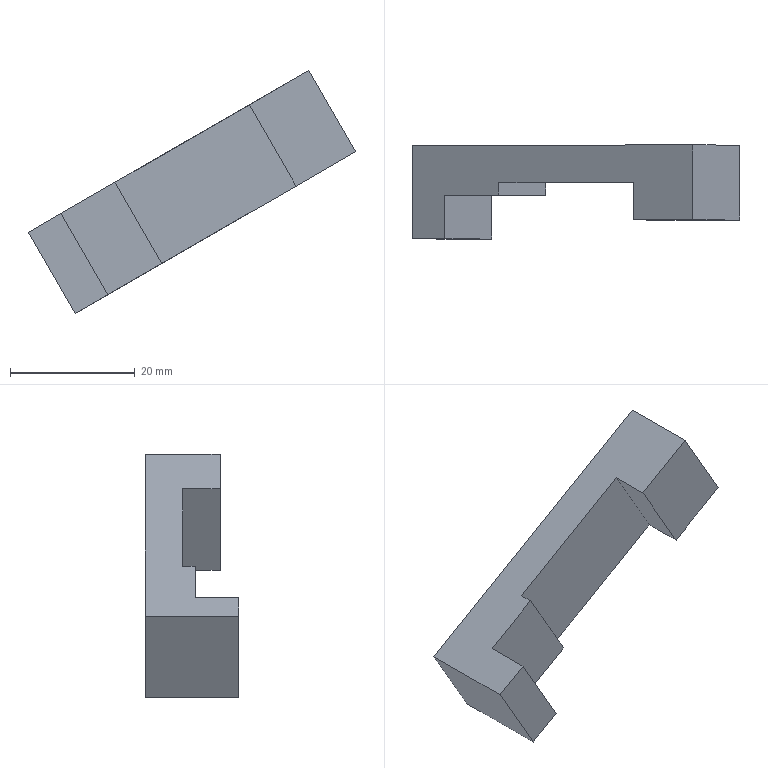Part | NX | features solid 2 | 1 solid | 12 faces | box 52.373 x 15 x 38.898 mm | volume 6763 mm3 | plane 12
STEP:
#1=CARTESIAN_POINT('',(16.962,778.,239.949));
#2=VERTEX_POINT('',#1);
#3=CARTESIAN_POINT('',(9.462,778.,252.94));
#4=VERTEX_POINT('',#3);
#5=CARTESIAN_POINT('',(16.962,778.,239.949));
#6=DIRECTION('',(0.5,0.,-0.866));
#7=VECTOR('',#6,1000.);
#8=LINE('',#5,#7);
#9=EDGE_CURVE('',#2,#4,#8,.F.);
#10=ORIENTED_EDGE('',*,*,#9,.T.);
#11=CARTESIAN_POINT('',(-12.029,778.,240.532));
#12=VERTEX_POINT('',#11);
#13=CARTESIAN_POINT('',(18.988,778.,258.44));
#14=DIRECTION('',(-0.866,0.,-0.5));
#15=VECTOR('',#14,1000.);
#16=LINE('',#13,#15);
#17=EDGE_CURVE('',#4,#12,#16,.T.);
#18=ORIENTED_EDGE('',*,*,#17,.T.);
#19=CARTESIAN_POINT('',(-4.529,778.,227.542));
#20=VERTEX_POINT('',#19);
#21=CARTESIAN_POINT('',(-4.529,778.,227.542));
#22=DIRECTION('',(-0.5,0.,0.866));
#23=VECTOR('',#22,1000.);
#24=LINE('',#21,#23);
#25=EDGE_CURVE('',#20,#12,#24,.T.);
#26=ORIENTED_EDGE('',*,*,#25,.F.);
#27=CARTESIAN_POINT('',(26.488,778.,245.449));
#28=DIRECTION('',(-0.866,0.,-0.5));
#29=VECTOR('',#28,1000.);
#30=LINE('',#27,#29);
#31=EDGE_CURVE('',#2,#20,#30,.T.);
#32=ORIENTED_EDGE('',*,*,#31,.F.);
#33=EDGE_LOOP('',(#10,#18,#26,#32));
#34=FACE_BOUND('',#33,.T.);
#35=CARTESIAN_POINT('',(11.488,778.,271.43));
#36=DIRECTION('',(0.,1.,0.));
#37=DIRECTION('',(-0.866,0.,-0.5));
#38=AXIS2_PLACEMENT_3D('',#35,#36,#37);
#39=PLANE('',#38);
#40=ADVANCED_FACE('',(#34),#39,.F.);
#41=CARTESIAN_POINT('',(26.488,784.,245.449));
#42=VERTEX_POINT('',#41);
#43=CARTESIAN_POINT('',(18.988,784.,258.44));
#44=VERTEX_POINT('',#43);
#45=CARTESIAN_POINT('',(11.488,784.,271.43));
#46=DIRECTION('',(0.5,0.,-0.866));
#47=VECTOR('',#46,1000.);
#48=LINE('',#45,#47);
#49=EDGE_CURVE('',#42,#44,#48,.F.);
#50=ORIENTED_EDGE('',*,*,#49,.F.);
#51=CARTESIAN_POINT('',(-18.385,784.,219.542));
#52=VERTEX_POINT('',#51);
#53=CARTESIAN_POINT('',(26.488,784.,245.449));
#54=DIRECTION('',(-0.866,0.,-0.5));
#55=VECTOR('',#54,1000.);
#56=LINE('',#53,#55);
#57=EDGE_CURVE('',#42,#52,#56,.T.);
#58=ORIENTED_EDGE('',*,*,#57,.T.);
#59=CARTESIAN_POINT('',(-25.885,784.,232.532));
#60=VERTEX_POINT('',#59);
#61=CARTESIAN_POINT('',(-33.385,784.,245.522));
#62=DIRECTION('',(-0.5,0.,0.866));
#63=VECTOR('',#62,1000.);
#64=LINE('',#61,#63);
#65=EDGE_CURVE('',#52,#60,#64,.T.);
#66=ORIENTED_EDGE('',*,*,#65,.T.);
#67=CARTESIAN_POINT('',(18.988,784.,258.44));
#68=DIRECTION('',(-0.866,0.,-0.5));
#69=VECTOR('',#68,1000.);
#70=LINE('',#67,#69);
#71=EDGE_CURVE('',#44,#60,#70,.T.);
#72=ORIENTED_EDGE('',*,*,#71,.F.);
#73=EDGE_LOOP('',(#50,#58,#66,#72));
#74=FACE_BOUND('',#73,.T.);
#75=CARTESIAN_POINT('',(11.488,784.,271.43));
#76=DIRECTION('',(0.,1.,0.));
#77=DIRECTION('',(-0.866,0.,-0.5));
#78=AXIS2_PLACEMENT_3D('',#75,#76,#77);
#79=PLANE('',#78);
#80=ADVANCED_FACE('',(#74),#79,.T.);
#81=ORIENTED_EDGE('',*,*,#65,.F.);
#82=CARTESIAN_POINT('',(-18.385,769.,219.542));
#83=VERTEX_POINT('',#82);
#84=CARTESIAN_POINT('',(-18.385,784.,219.542));
#85=DIRECTION('',(0.,1.,0.));
#86=VECTOR('',#85,1000.);
#87=LINE('',#84,#86);
#88=EDGE_CURVE('',#52,#83,#87,.F.);
#89=ORIENTED_EDGE('',*,*,#88,.T.);
#90=CARTESIAN_POINT('',(-25.885,769.,232.532));
#91=VERTEX_POINT('',#90);
#92=CARTESIAN_POINT('',(-18.385,769.,219.542));
#93=DIRECTION('',(-0.5,0.,0.866));
#94=VECTOR('',#93,1000.);
#95=LINE('',#92,#94);
#96=EDGE_CURVE('',#83,#91,#95,.T.);
#97=ORIENTED_EDGE('',*,*,#96,.T.);
#98=CARTESIAN_POINT('',(-25.885,784.,232.532));
#99=DIRECTION('',(0.,1.,0.));
#100=VECTOR('',#99,1000.);
#101=LINE('',#98,#100);
#102=EDGE_CURVE('',#60,#91,#101,.F.);
#103=ORIENTED_EDGE('',*,*,#102,.F.);
#104=EDGE_LOOP('',(#81,#89,#97,#103));
#105=FACE_BOUND('',#104,.T.);
#106=CARTESIAN_POINT('',(-33.385,784.,245.522));
#107=DIRECTION('',(-0.866,0.,-0.5));
#108=DIRECTION('',(0.,-1.,0.));
#109=AXIS2_PLACEMENT_3D('',#106,#107,#108);
#110=PLANE('',#109);
#111=ADVANCED_FACE('',(#105),#110,.T.);
#112=CARTESIAN_POINT('',(26.488,772.,245.449));
#113=VERTEX_POINT('',#112);
#114=CARTESIAN_POINT('',(26.488,784.,245.449));
#115=DIRECTION('',(0.,-1.,0.));
#116=VECTOR('',#115,1000.);
#117=LINE('',#114,#116);
#118=EDGE_CURVE('',#42,#113,#117,.T.);
#119=ORIENTED_EDGE('',*,*,#118,.F.);
#120=ORIENTED_EDGE('',*,*,#49,.T.);
#121=CARTESIAN_POINT('',(18.988,772.,258.44));
#122=VERTEX_POINT('',#121);
#123=CARTESIAN_POINT('',(18.988,784.,258.44));
#124=DIRECTION('',(0.,-1.,0.));
#125=VECTOR('',#124,1000.);
#126=LINE('',#123,#125);
#127=EDGE_CURVE('',#44,#122,#126,.T.);
#128=ORIENTED_EDGE('',*,*,#127,.T.);
#129=CARTESIAN_POINT('',(26.488,772.,245.449));
#130=DIRECTION('',(-0.5,0.,0.866));
#131=VECTOR('',#130,1000.);
#132=LINE('',#129,#131);
#133=EDGE_CURVE('',#113,#122,#132,.T.);
#134=ORIENTED_EDGE('',*,*,#133,.F.);
#135=EDGE_LOOP('',(#119,#120,#128,#134));
#136=FACE_BOUND('',#135,.T.);
#137=CARTESIAN_POINT('',(11.488,784.,271.43));
#138=DIRECTION('',(-0.866,0.,-0.5));
#139=DIRECTION('',(0.,-1.,0.));
#140=AXIS2_PLACEMENT_3D('',#137,#138,#139);
#141=PLANE('',#140);
#142=ADVANCED_FACE('',(#136),#141,.F.);
#143=CARTESIAN_POINT('',(-20.689,769.,235.532));
#144=VERTEX_POINT('',#143);
#145=CARTESIAN_POINT('',(-20.689,769.,235.532));
#146=DIRECTION('',(-0.866,0.,-0.5));
#147=VECTOR('',#146,1000.);
#148=LINE('',#145,#147);
#149=EDGE_CURVE('',#144,#91,#148,.T.);
#150=ORIENTED_EDGE('',*,*,#149,.F.);
#151=CARTESIAN_POINT('',(-20.689,776.,235.532));
#152=VERTEX_POINT('',#151);
#153=CARTESIAN_POINT('',(-20.689,778.,235.532));
#154=DIRECTION('',(0.,-1.,0.));
#155=VECTOR('',#154,1000.);
#156=LINE('',#153,#155);
#157=EDGE_CURVE('',#152,#144,#156,.T.);
#158=ORIENTED_EDGE('',*,*,#157,.F.);
#159=CARTESIAN_POINT('',(-12.029,776.,240.532));
#160=VERTEX_POINT('',#159);
#161=CARTESIAN_POINT('',(-12.029,776.,240.532));
#162=DIRECTION('',(-0.866,0.,-0.5));
#163=VECTOR('',#162,1000.);
#164=LINE('',#161,#163);
#165=EDGE_CURVE('',#160,#152,#164,.T.);
#166=ORIENTED_EDGE('',*,*,#165,.F.);
#167=CARTESIAN_POINT('',(-12.029,778.,240.532));
#168=DIRECTION('',(0.,-1.,0.));
#169=VECTOR('',#168,1000.);
#170=LINE('',#167,#169);
#171=EDGE_CURVE('',#12,#160,#170,.T.);
#172=ORIENTED_EDGE('',*,*,#171,.F.);
#173=ORIENTED_EDGE('',*,*,#17,.F.);
#174=CARTESIAN_POINT('',(9.462,772.,252.94));
#175=VERTEX_POINT('',#174);
#176=CARTESIAN_POINT('',(9.462,772.,252.94));
#177=DIRECTION('',(0.,-1.,0.));
#178=VECTOR('',#177,1000.);
#179=LINE('',#176,#178);
#180=EDGE_CURVE('',#175,#4,#179,.F.);
#181=ORIENTED_EDGE('',*,*,#180,.F.);
#182=CARTESIAN_POINT('',(18.988,772.,258.44));
#183=DIRECTION('',(0.866,0.,0.5));
#184=VECTOR('',#183,1000.);
#185=LINE('',#182,#184);
#186=EDGE_CURVE('',#122,#175,#185,.F.);
#187=ORIENTED_EDGE('',*,*,#186,.F.);
#188=ORIENTED_EDGE('',*,*,#127,.F.);
#189=ORIENTED_EDGE('',*,*,#71,.T.);
#190=ORIENTED_EDGE('',*,*,#102,.T.);
#191=EDGE_LOOP('',(#150,#158,#166,#172,#173,#181,#187,#188,#189,#190));
#192=FACE_BOUND('',#191,.T.);
#193=CARTESIAN_POINT('',(18.988,784.,258.44));
#194=DIRECTION('',(0.5,0.,-0.866));
#195=DIRECTION('',(-0.866,0.,-0.5));
#196=AXIS2_PLACEMENT_3D('',#193,#194,#195);
#197=PLANE('',#196);
#198=ADVANCED_FACE('',(#192),#197,.F.);
#199=ORIENTED_EDGE('',*,*,#88,.F.);
#200=ORIENTED_EDGE('',*,*,#57,.F.);
#201=ORIENTED_EDGE('',*,*,#118,.T.);
#202=CARTESIAN_POINT('',(16.962,772.,239.949));
#203=VERTEX_POINT('',#202);
#204=CARTESIAN_POINT('',(26.488,772.,245.449));
#205=DIRECTION('',(0.866,0.,0.5));
#206=VECTOR('',#205,1000.);
#207=LINE('',#204,#206);
#208=EDGE_CURVE('',#113,#203,#207,.F.);
#209=ORIENTED_EDGE('',*,*,#208,.T.);
#210=CARTESIAN_POINT('',(16.962,772.,239.949));
#211=DIRECTION('',(0.,-1.,0.));
#212=VECTOR('',#211,1000.);
#213=LINE('',#210,#212);
#214=EDGE_CURVE('',#203,#2,#213,.F.);
#215=ORIENTED_EDGE('',*,*,#214,.T.);
#216=ORIENTED_EDGE('',*,*,#31,.T.);
#217=CARTESIAN_POINT('',(-4.529,776.,227.542));
#218=VERTEX_POINT('',#217);
#219=CARTESIAN_POINT('',(-4.529,778.,227.542));
#220=DIRECTION('',(0.,-1.,0.));
#221=VECTOR('',#220,1000.);
#222=LINE('',#219,#221);
#223=EDGE_CURVE('',#20,#218,#222,.T.);
#224=ORIENTED_EDGE('',*,*,#223,.T.);
#225=CARTESIAN_POINT('',(-13.189,776.,222.542));
#226=VERTEX_POINT('',#225);
#227=CARTESIAN_POINT('',(-4.529,776.,227.542));
#228=DIRECTION('',(-0.866,0.,-0.5));
#229=VECTOR('',#228,1000.);
#230=LINE('',#227,#229);
#231=EDGE_CURVE('',#218,#226,#230,.T.);
#232=ORIENTED_EDGE('',*,*,#231,.T.);
#233=CARTESIAN_POINT('',(-13.189,769.,222.542));
#234=VERTEX_POINT('',#233);
#235=CARTESIAN_POINT('',(-13.189,778.,222.542));
#236=DIRECTION('',(0.,-1.,0.));
#237=VECTOR('',#236,1000.);
#238=LINE('',#235,#237);
#239=EDGE_CURVE('',#226,#234,#238,.T.);
#240=ORIENTED_EDGE('',*,*,#239,.T.);
#241=CARTESIAN_POINT('',(-13.189,769.,222.542));
#242=DIRECTION('',(-0.866,0.,-0.5));
#243=VECTOR('',#242,1000.);
#244=LINE('',#241,#243);
#245=EDGE_CURVE('',#234,#83,#244,.T.);
#246=ORIENTED_EDGE('',*,*,#245,.T.);
#247=EDGE_LOOP('',(#199,#200,#201,#209,#215,#216,#224,#232,#240,#246));
#248=FACE_BOUND('',#247,.T.);
#249=CARTESIAN_POINT('',(26.488,784.,245.449));
#250=DIRECTION('',(0.5,0.,-0.866));
#251=DIRECTION('',(-0.866,0.,-0.5));
#252=AXIS2_PLACEMENT_3D('',#249,#250,#251);
#253=PLANE('',#252);
#254=ADVANCED_FACE('',(#248),#253,.T.);
#255=ORIENTED_EDGE('',*,*,#171,.T.);
#256=CARTESIAN_POINT('',(-4.529,776.,227.542));
#257=DIRECTION('',(-0.5,0.,0.866));
#258=VECTOR('',#257,1000.);
#259=LINE('',#256,#258);
#260=EDGE_CURVE('',#218,#160,#259,.T.);
#261=ORIENTED_EDGE('',*,*,#260,.F.);
#262=ORIENTED_EDGE('',*,*,#223,.F.);
#263=ORIENTED_EDGE('',*,*,#25,.T.);
#264=EDGE_LOOP('',(#255,#261,#262,#263));
#265=FACE_BOUND('',#264,.T.);
#266=CARTESIAN_POINT('',(-4.529,778.,227.542));
#267=DIRECTION('',(0.866,0.,0.5));
#268=DIRECTION('',(-0.5,0.,0.866));
#269=AXIS2_PLACEMENT_3D('',#266,#267,#268);
#270=PLANE('',#269);
#271=ADVANCED_FACE('',(#265),#270,.T.);
#272=CARTESIAN_POINT('',(-13.189,776.,222.542));
#273=DIRECTION('',(-0.5,0.,0.866));
#274=VECTOR('',#273,1000.);
#275=LINE('',#272,#274);
#276=EDGE_CURVE('',#226,#152,#275,.T.);
#277=ORIENTED_EDGE('',*,*,#276,.F.);
#278=ORIENTED_EDGE('',*,*,#231,.F.);
#279=ORIENTED_EDGE('',*,*,#260,.T.);
#280=ORIENTED_EDGE('',*,*,#165,.T.);
#281=EDGE_LOOP('',(#277,#278,#279,#280));
#282=FACE_BOUND('',#281,.T.);
#283=CARTESIAN_POINT('',(-4.529,776.,227.542));
#284=DIRECTION('',(0.,1.,0.));
#285=DIRECTION('',(0.,0.,-1.));
#286=AXIS2_PLACEMENT_3D('',#283,#284,#285);
#287=PLANE('',#286);
#288=ADVANCED_FACE('',(#282),#287,.F.);
#289=ORIENTED_EDGE('',*,*,#276,.T.);
#290=ORIENTED_EDGE('',*,*,#157,.T.);
#291=CARTESIAN_POINT('',(-13.189,769.,222.542));
#292=DIRECTION('',(-0.5,0.,0.866));
#293=VECTOR('',#292,1000.);
#294=LINE('',#291,#293);
#295=EDGE_CURVE('',#234,#144,#294,.T.);
#296=ORIENTED_EDGE('',*,*,#295,.F.);
#297=ORIENTED_EDGE('',*,*,#239,.F.);
#298=EDGE_LOOP('',(#289,#290,#296,#297));
#299=FACE_BOUND('',#298,.T.);
#300=CARTESIAN_POINT('',(-13.189,778.,222.542));
#301=DIRECTION('',(0.866,0.,0.5));
#302=DIRECTION('',(-0.5,0.,0.866));
#303=AXIS2_PLACEMENT_3D('',#300,#301,#302);
#304=PLANE('',#303);
#305=ADVANCED_FACE('',(#299),#304,.T.);
#306=ORIENTED_EDGE('',*,*,#96,.F.);
#307=ORIENTED_EDGE('',*,*,#245,.F.);
#308=ORIENTED_EDGE('',*,*,#295,.T.);
#309=ORIENTED_EDGE('',*,*,#149,.T.);
#310=EDGE_LOOP('',(#306,#307,#308,#309));
#311=FACE_BOUND('',#310,.T.);
#312=CARTESIAN_POINT('',(-13.189,769.,222.542));
#313=DIRECTION('',(0.,1.,0.));
#314=DIRECTION('',(0.,0.,-1.));
#315=AXIS2_PLACEMENT_3D('',#312,#313,#314);
#316=PLANE('',#315);
#317=ADVANCED_FACE('',(#311),#316,.F.);
#318=ORIENTED_EDGE('',*,*,#208,.F.);
#319=ORIENTED_EDGE('',*,*,#133,.T.);
#320=ORIENTED_EDGE('',*,*,#186,.T.);
#321=CARTESIAN_POINT('',(16.962,772.,239.949));
#322=DIRECTION('',(0.5,0.,-0.866));
#323=VECTOR('',#322,1000.);
#324=LINE('',#321,#323);
#325=EDGE_CURVE('',#203,#175,#324,.F.);
#326=ORIENTED_EDGE('',*,*,#325,.F.);
#327=EDGE_LOOP('',(#318,#319,#320,#326));
#328=FACE_BOUND('',#327,.T.);
#329=CARTESIAN_POINT('',(26.488,772.,245.449));
#330=DIRECTION('',(0.,-1.,0.));
#331=DIRECTION('',(-0.5,0.,0.866));
#332=AXIS2_PLACEMENT_3D('',#329,#330,#331);
#333=PLANE('',#332);
#334=ADVANCED_FACE('',(#328),#333,.T.);
#335=ORIENTED_EDGE('',*,*,#9,.F.);
#336=ORIENTED_EDGE('',*,*,#214,.F.);
#337=ORIENTED_EDGE('',*,*,#325,.T.);
#338=ORIENTED_EDGE('',*,*,#180,.T.);
#339=EDGE_LOOP('',(#335,#336,#337,#338));
#340=FACE_BOUND('',#339,.T.);
#341=CARTESIAN_POINT('',(16.962,772.,239.949));
#342=DIRECTION('',(0.866,0.,0.5));
#343=DIRECTION('',(0.5,0.,-0.866));
#344=AXIS2_PLACEMENT_3D('',#341,#342,#343);
#345=PLANE('',#344);
#346=ADVANCED_FACE('',(#340),#345,.F.);
#347=CLOSED_SHELL('',(#40,#80,#111,#142,#198,#254,#271,#288,#305,#317,#334,#346));
#348=MANIFOLD_SOLID_BREP('',#347);
#349=(LENGTH_UNIT()NAMED_UNIT(*)SI_UNIT(.MILLI.,.METRE.));
#350=UNCERTAINTY_MEASURE_WITH_UNIT(LENGTH_MEASURE(0.00001),#349,'','');
#351=(NAMED_UNIT(*)PLANE_ANGLE_UNIT()SI_UNIT($,.RADIAN.));
#352=(NAMED_UNIT(*)SI_UNIT($,.STERADIAN.)SOLID_ANGLE_UNIT());
#353=(GEOMETRIC_REPRESENTATION_CONTEXT(3)GLOBAL_UNCERTAINTY_ASSIGNED_CONTEXT((#350))GLOBAL_UNIT_ASSIGNED_CONTEXT((#349,#351,#352))REPRESENTATION_CONTEXT('',''));
#354=ADVANCED_BREP_SHAPE_REPRESENTATION('',(#348),#353);